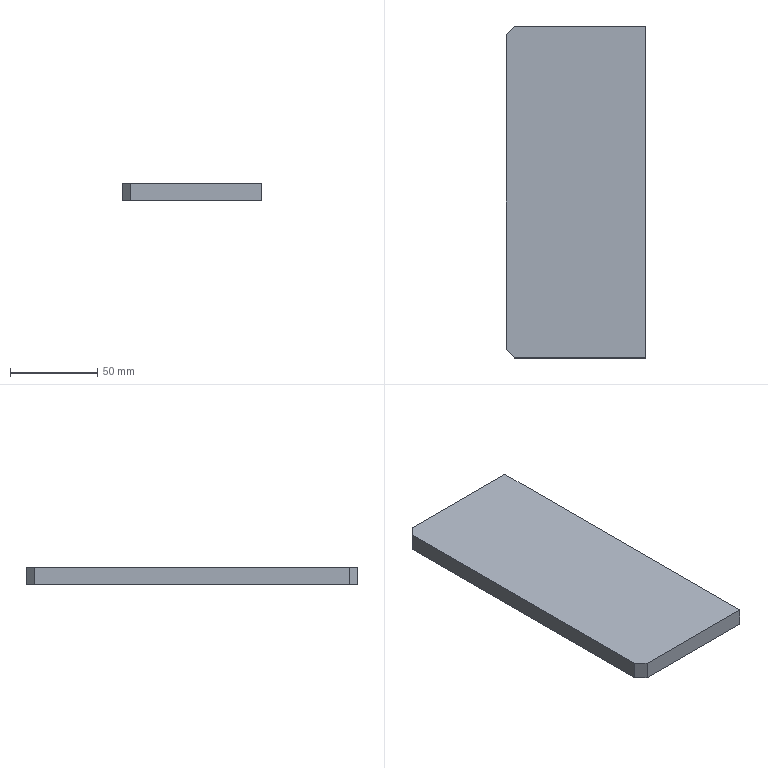Part | STEP file | Main beam baffle 2 | 1 solid | 8 faces | box 80 x 190 x 10 mm | volume 151750 mm3 | plane 8
STEP:
#1=CARTESIAN_POINT('',(40.,-95.,0.));
#2=VERTEX_POINT('',#1);
#3=CARTESIAN_POINT('',(40.,95.,0.));
#4=VERTEX_POINT('',#3);
#5=CARTESIAN_POINT('',(40.,95.,0.));
#6=DIRECTION('',(0.,1.,0.));
#7=VECTOR('',#6,1000.);
#8=LINE('',#5,#7);
#9=EDGE_CURVE('',#2,#4,#8,.T.);
#10=ORIENTED_EDGE('',*,*,#9,.T.);
#11=CARTESIAN_POINT('',(40.,95.,10.));
#12=VERTEX_POINT('',#11);
#13=CARTESIAN_POINT('',(40.,95.,10.));
#14=DIRECTION('',(0.,0.,-1.));
#15=VECTOR('',#14,1000.);
#16=LINE('',#13,#15);
#17=EDGE_CURVE('',#12,#4,#16,.T.);
#18=ORIENTED_EDGE('',*,*,#17,.F.);
#19=CARTESIAN_POINT('',(40.,-95.,10.));
#20=VERTEX_POINT('',#19);
#21=CARTESIAN_POINT('',(40.,95.,10.));
#22=DIRECTION('',(0.,1.,0.));
#23=VECTOR('',#22,1000.);
#24=LINE('',#21,#23);
#25=EDGE_CURVE('',#20,#12,#24,.T.);
#26=ORIENTED_EDGE('',*,*,#25,.F.);
#27=CARTESIAN_POINT('',(40.,-95.,10.));
#28=DIRECTION('',(0.,0.,-1.));
#29=VECTOR('',#28,1000.);
#30=LINE('',#27,#29);
#31=EDGE_CURVE('',#20,#2,#30,.T.);
#32=ORIENTED_EDGE('',*,*,#31,.T.);
#33=EDGE_LOOP('',(#10,#18,#26,#32));
#34=FACE_OUTER_BOUND('',#33,.T.);
#35=CARTESIAN_POINT('',(40.,95.,10.));
#36=DIRECTION('',(-1.,0.,0.));
#37=DIRECTION('',(0.,-1.,0.));
#38=AXIS2_PLACEMENT_3D('',#35,#36,#37);
#39=PLANE('',#38);
#40=ADVANCED_FACE('',(#34),#39,.F.);
#41=CARTESIAN_POINT('',(-35.,95.,0.));
#42=VERTEX_POINT('',#41);
#43=CARTESIAN_POINT('',(-40.,95.,0.));
#44=DIRECTION('',(-1.,0.,0.));
#45=VECTOR('',#44,1000.);
#46=LINE('',#43,#45);
#47=EDGE_CURVE('',#4,#42,#46,.T.);
#48=ORIENTED_EDGE('',*,*,#47,.T.);
#49=CARTESIAN_POINT('',(-35.,95.,10.));
#50=VERTEX_POINT('',#49);
#51=CARTESIAN_POINT('',(-35.,95.,10.));
#52=DIRECTION('',(0.,0.,1.));
#53=VECTOR('',#52,1000.);
#54=LINE('',#51,#53);
#55=EDGE_CURVE('',#42,#50,#54,.T.);
#56=ORIENTED_EDGE('',*,*,#55,.T.);
#57=CARTESIAN_POINT('',(-40.,95.,10.));
#58=DIRECTION('',(-1.,0.,0.));
#59=VECTOR('',#58,1000.);
#60=LINE('',#57,#59);
#61=EDGE_CURVE('',#12,#50,#60,.T.);
#62=ORIENTED_EDGE('',*,*,#61,.F.);
#63=ORIENTED_EDGE('',*,*,#17,.T.);
#64=EDGE_LOOP('',(#48,#56,#62,#63));
#65=FACE_OUTER_BOUND('',#64,.T.);
#66=CARTESIAN_POINT('',(-40.,95.,10.));
#67=DIRECTION('',(0.,-1.,0.));
#68=DIRECTION('',(0.,0.,-1.));
#69=AXIS2_PLACEMENT_3D('',#66,#67,#68);
#70=PLANE('',#69);
#71=ADVANCED_FACE('',(#65),#70,.F.);
#72=CARTESIAN_POINT('',(-40.,90.,0.));
#73=VERTEX_POINT('',#72);
#74=CARTESIAN_POINT('',(-40.,-90.,0.));
#75=VERTEX_POINT('',#74);
#76=CARTESIAN_POINT('',(-40.,95.,0.));
#77=DIRECTION('',(0.,-1.,0.));
#78=VECTOR('',#77,1000.);
#79=LINE('',#76,#78);
#80=EDGE_CURVE('',#73,#75,#79,.T.);
#81=ORIENTED_EDGE('',*,*,#80,.T.);
#82=CARTESIAN_POINT('',(-40.,-90.,10.));
#83=VERTEX_POINT('',#82);
#84=CARTESIAN_POINT('',(-40.,-90.,10.));
#85=DIRECTION('',(0.,0.,1.));
#86=VECTOR('',#85,1000.);
#87=LINE('',#84,#86);
#88=EDGE_CURVE('',#75,#83,#87,.T.);
#89=ORIENTED_EDGE('',*,*,#88,.T.);
#90=CARTESIAN_POINT('',(-40.,90.,10.));
#91=VERTEX_POINT('',#90);
#92=CARTESIAN_POINT('',(-40.,95.,10.));
#93=DIRECTION('',(0.,-1.,0.));
#94=VECTOR('',#93,1000.);
#95=LINE('',#92,#94);
#96=EDGE_CURVE('',#91,#83,#95,.T.);
#97=ORIENTED_EDGE('',*,*,#96,.F.);
#98=CARTESIAN_POINT('',(-40.,90.,10.));
#99=DIRECTION('',(0.,0.,-1.));
#100=VECTOR('',#99,1000.);
#101=LINE('',#98,#100);
#102=EDGE_CURVE('',#91,#73,#101,.T.);
#103=ORIENTED_EDGE('',*,*,#102,.T.);
#104=EDGE_LOOP('',(#81,#89,#97,#103));
#105=FACE_OUTER_BOUND('',#104,.T.);
#106=CARTESIAN_POINT('',(-40.,95.,10.));
#107=DIRECTION('',(1.,0.,0.));
#108=DIRECTION('',(0.,1.,0.));
#109=AXIS2_PLACEMENT_3D('',#106,#107,#108);
#110=PLANE('',#109);
#111=ADVANCED_FACE('',(#105),#110,.F.);
#112=CARTESIAN_POINT('',(-35.,-95.,10.));
#113=VERTEX_POINT('',#112);
#114=CARTESIAN_POINT('',(-40.,-95.,10.));
#115=DIRECTION('',(1.,0.,0.));
#116=VECTOR('',#115,1000.);
#117=LINE('',#114,#116);
#118=EDGE_CURVE('',#113,#20,#117,.T.);
#119=ORIENTED_EDGE('',*,*,#118,.F.);
#120=CARTESIAN_POINT('',(-35.,-95.,0.));
#121=VERTEX_POINT('',#120);
#122=CARTESIAN_POINT('',(-35.,-95.,10.));
#123=DIRECTION('',(0.,0.,-1.));
#124=VECTOR('',#123,1000.);
#125=LINE('',#122,#124);
#126=EDGE_CURVE('',#113,#121,#125,.T.);
#127=ORIENTED_EDGE('',*,*,#126,.T.);
#128=CARTESIAN_POINT('',(-40.,-95.,0.));
#129=DIRECTION('',(1.,0.,0.));
#130=VECTOR('',#129,1000.);
#131=LINE('',#128,#130);
#132=EDGE_CURVE('',#121,#2,#131,.T.);
#133=ORIENTED_EDGE('',*,*,#132,.T.);
#134=ORIENTED_EDGE('',*,*,#31,.F.);
#135=EDGE_LOOP('',(#119,#127,#133,#134));
#136=FACE_OUTER_BOUND('',#135,.T.);
#137=CARTESIAN_POINT('',(-40.,-95.,10.));
#138=DIRECTION('',(0.,1.,0.));
#139=DIRECTION('',(0.,0.,1.));
#140=AXIS2_PLACEMENT_3D('',#137,#138,#139);
#141=PLANE('',#140);
#142=ADVANCED_FACE('',(#136),#141,.F.);
#143=ORIENTED_EDGE('',*,*,#96,.T.);
#144=CARTESIAN_POINT('',(-65.,-65.,10.));
#145=DIRECTION('',(0.7071,-0.7071,0.));
#146=VECTOR('',#145,1000.);
#147=LINE('',#144,#146);
#148=EDGE_CURVE('',#83,#113,#147,.T.);
#149=ORIENTED_EDGE('',*,*,#148,.T.);
#150=ORIENTED_EDGE('',*,*,#118,.T.);
#151=ORIENTED_EDGE('',*,*,#25,.T.);
#152=ORIENTED_EDGE('',*,*,#61,.T.);
#153=CARTESIAN_POINT('',(-65.,65.,10.));
#154=DIRECTION('',(-0.7071,-0.7071,0.));
#155=VECTOR('',#154,1000.);
#156=LINE('',#153,#155);
#157=EDGE_CURVE('',#50,#91,#156,.T.);
#158=ORIENTED_EDGE('',*,*,#157,.T.);
#159=EDGE_LOOP('',(#143,#149,#150,#151,#152,#158));
#160=FACE_OUTER_BOUND('',#159,.T.);
#161=CARTESIAN_POINT('',(0.,0.,10.));
#162=DIRECTION('',(0.,0.,1.));
#163=DIRECTION('',(1.,0.,0.));
#164=AXIS2_PLACEMENT_3D('',#161,#162,#163);
#165=PLANE('',#164);
#166=ADVANCED_FACE('',(#160),#165,.T.);
#167=ORIENTED_EDGE('',*,*,#132,.F.);
#168=CARTESIAN_POINT('',(-35.,-95.,0.));
#169=DIRECTION('',(-0.7071,0.7071,0.));
#170=VECTOR('',#169,1000.);
#171=LINE('',#168,#170);
#172=EDGE_CURVE('',#121,#75,#171,.T.);
#173=ORIENTED_EDGE('',*,*,#172,.T.);
#174=ORIENTED_EDGE('',*,*,#80,.F.);
#175=CARTESIAN_POINT('',(-40.,90.,0.));
#176=DIRECTION('',(0.7071,0.7071,0.));
#177=VECTOR('',#176,1000.);
#178=LINE('',#175,#177);
#179=EDGE_CURVE('',#73,#42,#178,.T.);
#180=ORIENTED_EDGE('',*,*,#179,.T.);
#181=ORIENTED_EDGE('',*,*,#47,.F.);
#182=ORIENTED_EDGE('',*,*,#9,.F.);
#183=EDGE_LOOP('',(#167,#173,#174,#180,#181,#182));
#184=FACE_OUTER_BOUND('',#183,.T.);
#185=CARTESIAN_POINT('',(0.,0.,0.));
#186=DIRECTION('',(0.,0.,1.));
#187=DIRECTION('',(1.,0.,0.));
#188=AXIS2_PLACEMENT_3D('',#185,#186,#187);
#189=PLANE('',#188);
#190=ADVANCED_FACE('',(#184),#189,.F.);
#191=ORIENTED_EDGE('',*,*,#148,.F.);
#192=ORIENTED_EDGE('',*,*,#88,.F.);
#193=ORIENTED_EDGE('',*,*,#172,.F.);
#194=ORIENTED_EDGE('',*,*,#126,.F.);
#195=EDGE_LOOP('',(#191,#192,#193,#194));
#196=FACE_OUTER_BOUND('',#195,.T.);
#197=CARTESIAN_POINT('',(-35.,-95.,10.));
#198=DIRECTION('',(0.7071,0.7071,0.));
#199=DIRECTION('',(0.,0.,-1.));
#200=AXIS2_PLACEMENT_3D('',#197,#198,#199);
#201=PLANE('',#200);
#202=ADVANCED_FACE('',(#196),#201,.F.);
#203=ORIENTED_EDGE('',*,*,#157,.F.);
#204=ORIENTED_EDGE('',*,*,#55,.F.);
#205=ORIENTED_EDGE('',*,*,#179,.F.);
#206=ORIENTED_EDGE('',*,*,#102,.F.);
#207=EDGE_LOOP('',(#203,#204,#205,#206));
#208=FACE_OUTER_BOUND('',#207,.T.);
#209=CARTESIAN_POINT('',(-40.,90.,10.));
#210=DIRECTION('',(0.7071,-0.7071,0.));
#211=DIRECTION('',(0.,0.,-1.));
#212=AXIS2_PLACEMENT_3D('',#209,#210,#211);
#213=PLANE('',#212);
#214=ADVANCED_FACE('',(#208),#213,.F.);
#215=CLOSED_SHELL('',(#40,#71,#111,#142,#166,#190,#202,#214));
#216=MANIFOLD_SOLID_BREP('',#215);
#217=CARTESIAN_POINT('',(0.,0.,0.));
#218=DIRECTION('',(0.,0.,1.));
#219=DIRECTION('',(1.,0.,0.));
#220=AXIS2_PLACEMENT_3D('',#217,#218,#219);
#221=(LENGTH_UNIT()NAMED_UNIT(*)SI_UNIT(.MILLI.,.METRE.));
#222=UNCERTAINTY_MEASURE_WITH_UNIT(LENGTH_MEASURE(0.00001),#221,'','');
#223=(NAMED_UNIT(*)PLANE_ANGLE_UNIT()SI_UNIT($,.RADIAN.));
#224=(NAMED_UNIT(*)SI_UNIT($,.STERADIAN.)SOLID_ANGLE_UNIT());
#225=(GEOMETRIC_REPRESENTATION_CONTEXT(3)GLOBAL_UNCERTAINTY_ASSIGNED_CONTEXT((#222))GLOBAL_UNIT_ASSIGNED_CONTEXT((#221,#223,#224))REPRESENTATION_CONTEXT('',''));
#226=ADVANCED_BREP_SHAPE_REPRESENTATION('',(#216,#220),#225);